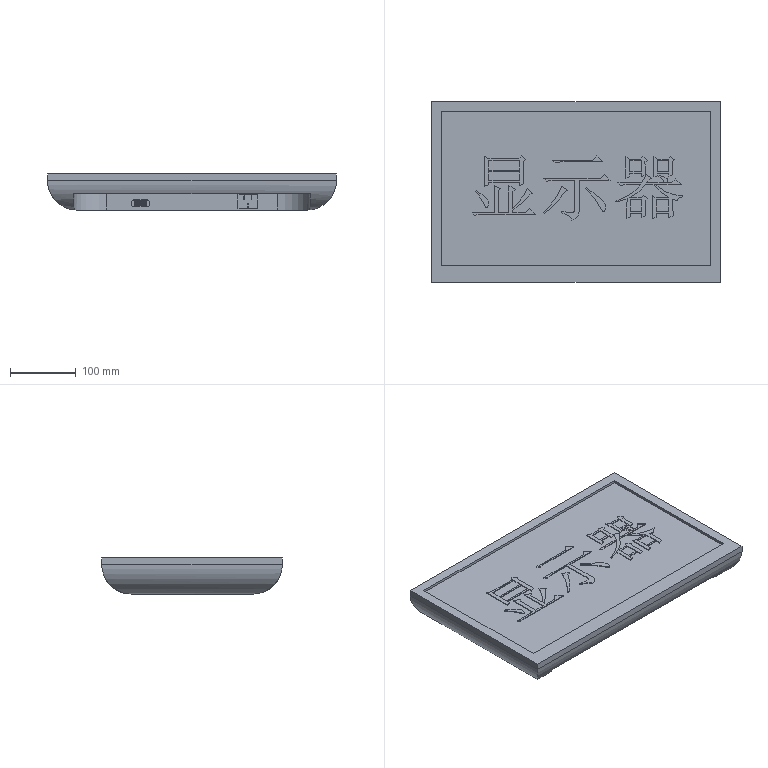Part | STEP file | Guide wheel mechanism revised.sldasm-Part-313 | 1 solid | 368 faces | box 440 x 275 x 55 mm | volume 5174621 mm3 | plane 213 | cylinder 113 | spline 34 | cone 8 | commonest cylinder face diameters 0.886 x80 1 x9 3.3 x8 4.6 x8 90 x4 10.793 x2